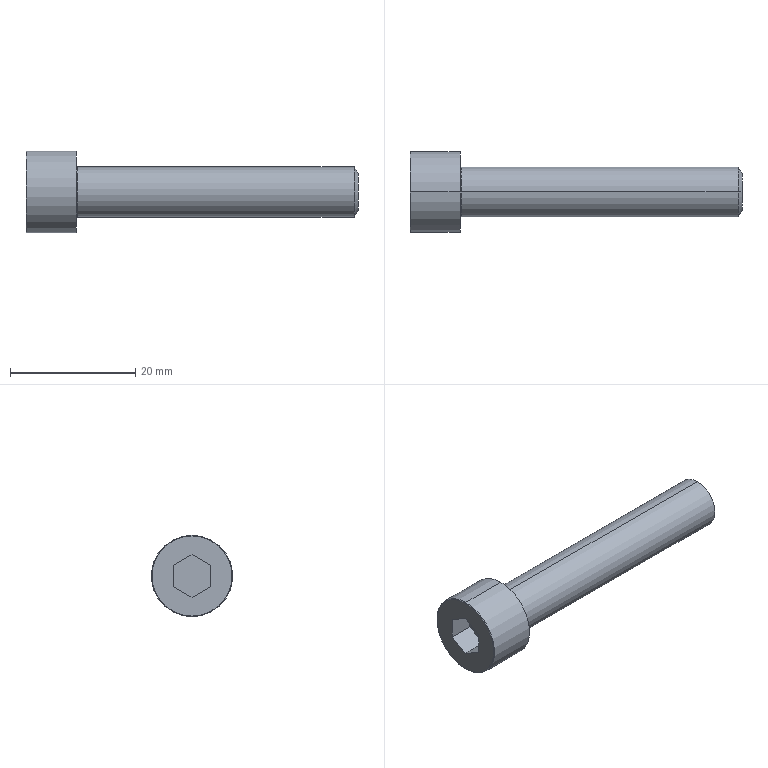Part | SolidWorks | features BlendCut 1, Cut 1, Fillet 1, LPattern 1, RevCut 1, Revolution 1 | 1 solid | 20 faces | box 53 x 13 x 13 mm | volume 3194 mm3 | plane 10 | torus 4 | cylinder 4 | cone 2 | commonest cylinder face diameters 8 x2 13 x2
STEP:
#1=CARTESIAN_POINT('',(0.,0.,6.4));
#2=VERTEX_POINT('',#1);
#3=CARTESIAN_POINT('',(0.,0.,-6.4));
#4=VERTEX_POINT('',#3);
#5=CARTESIAN_POINT('',(0.,0.,0.));
#6=DIRECTION('',(-1.,0.,0.));
#7=DIRECTION('',(0.,0.,-1.));
#8=AXIS2_PLACEMENT_3D('',#5,#6,#7);
#9=CIRCLE('',#8,6.4);
#10=EDGE_CURVE('',#2,#4,#9,.T.);
#11=ORIENTED_EDGE('',*,*,#10,.F.);
#12=CARTESIAN_POINT('',(0.1,0.,6.5));
#13=VERTEX_POINT('',#12);
#14=CARTESIAN_POINT('',(0.1,0.,6.4));
#15=DIRECTION('',(0.,1.,0.));
#16=DIRECTION('',(0.,0.,1.));
#17=AXIS2_PLACEMENT_3D('',#14,#15,#16);
#18=CIRCLE('',#17,0.1);
#19=EDGE_CURVE('',#2,#13,#18,.T.);
#20=ORIENTED_EDGE('',*,*,#19,.T.);
#21=CARTESIAN_POINT('',(0.1,0.,-6.5));
#22=VERTEX_POINT('',#21);
#23=CARTESIAN_POINT('',(0.1,0.,0.));
#24=DIRECTION('',(1.,0.,0.));
#25=DIRECTION('',(0.,0.,-1.));
#26=AXIS2_PLACEMENT_3D('',#23,#24,#25);
#27=CIRCLE('',#26,6.5);
#28=EDGE_CURVE('',#22,#13,#27,.T.);
#29=ORIENTED_EDGE('',*,*,#28,.F.);
#30=CARTESIAN_POINT('',(0.1,0.,-6.4));
#31=DIRECTION('',(0.,-1.,0.));
#32=DIRECTION('',(0.,0.,-1.));
#33=AXIS2_PLACEMENT_3D('',#30,#31,#32);
#34=CIRCLE('',#33,0.1);
#35=EDGE_CURVE('',#4,#22,#34,.T.);
#36=ORIENTED_EDGE('',*,*,#35,.F.);
#37=EDGE_LOOP('',(#11,#20,#29,#36));
#38=FACE_OUTER_BOUND('',#37,.T.);
#39=CARTESIAN_POINT('',(0.1,0.,0.));
#40=DIRECTION('',(1.,0.,0.));
#41=DIRECTION('',(0.,0.,-1.));
#42=AXIS2_PLACEMENT_3D('',#39,#40,#41);
#43=TOROIDAL_SURFACE('',#42,6.4,0.1);
#44=ADVANCED_FACE('',(#38),#43,.T.);
#45=CARTESIAN_POINT('',(53.,0.,2.917));
#46=VERTEX_POINT('',#45);
#47=CARTESIAN_POINT('',(53.,0.,-2.917));
#48=VERTEX_POINT('',#47);
#49=CARTESIAN_POINT('',(53.,0.,0.));
#50=DIRECTION('',(-1.,0.,0.));
#51=DIRECTION('',(0.,0.,1.));
#52=AXIS2_PLACEMENT_3D('',#49,#50,#51);
#53=CIRCLE('',#52,2.917);
#54=EDGE_CURVE('',#46,#48,#53,.T.);
#55=ORIENTED_EDGE('',*,*,#54,.T.);
#56=CARTESIAN_POINT('',(52.375,0.,-4.));
#57=VERTEX_POINT('',#56);
#58=CARTESIAN_POINT('',(52.375,0.,-4.));
#59=DIRECTION('',(-0.5,0.,-0.866));
#60=VECTOR('',#59,1000.);
#61=LINE('',#58,#60);
#62=EDGE_CURVE('',#48,#57,#61,.T.);
#63=ORIENTED_EDGE('',*,*,#62,.T.);
#64=CARTESIAN_POINT('',(52.375,0.,4.));
#65=VERTEX_POINT('',#64);
#66=CARTESIAN_POINT('',(52.375,0.,0.));
#67=DIRECTION('',(-1.,0.,0.));
#68=DIRECTION('',(0.,0.,1.));
#69=AXIS2_PLACEMENT_3D('',#66,#67,#68);
#70=CIRCLE('',#69,4.);
#71=EDGE_CURVE('',#65,#57,#70,.T.);
#72=ORIENTED_EDGE('',*,*,#71,.F.);
#73=CARTESIAN_POINT('',(52.375,0.,4.));
#74=DIRECTION('',(-0.5,0.,0.866));
#75=VECTOR('',#74,1000.);
#76=LINE('',#73,#75);
#77=EDGE_CURVE('',#46,#65,#76,.T.);
#78=ORIENTED_EDGE('',*,*,#77,.F.);
#79=EDGE_LOOP('',(#55,#63,#72,#78));
#80=FACE_OUTER_BOUND('',#79,.T.);
#81=CARTESIAN_POINT('',(52.375,0.,0.));
#82=DIRECTION('',(-1.,0.,0.));
#83=DIRECTION('',(0.,0.,1.));
#84=AXIS2_PLACEMENT_3D('',#81,#82,#83);
#85=CONICAL_SURFACE('',#84,4.,1.047);
#86=ADVANCED_FACE('',(#80),#85,.T.);
#87=CARTESIAN_POINT('',(8.,0.,-4.2));
#88=VERTEX_POINT('',#87);
#89=CARTESIAN_POINT('',(8.,0.,4.2));
#90=VERTEX_POINT('',#89);
#91=CARTESIAN_POINT('',(8.,0.,0.));
#92=DIRECTION('',(-1.,0.,0.));
#93=DIRECTION('',(0.,0.,1.));
#94=AXIS2_PLACEMENT_3D('',#91,#92,#93);
#95=CIRCLE('',#94,4.2);
#96=EDGE_CURVE('',#88,#90,#95,.T.);
#97=ORIENTED_EDGE('',*,*,#96,.F.);
#98=CARTESIAN_POINT('',(8.2,0.,-4.));
#99=VERTEX_POINT('',#98);
#100=CARTESIAN_POINT('',(8.2,0.,-4.2));
#101=DIRECTION('',(0.,1.,0.));
#102=DIRECTION('',(0.,0.,1.));
#103=AXIS2_PLACEMENT_3D('',#100,#101,#102);
#104=CIRCLE('',#103,0.2);
#105=EDGE_CURVE('',#88,#99,#104,.T.);
#106=ORIENTED_EDGE('',*,*,#105,.T.);
#107=CARTESIAN_POINT('',(8.2,0.,4.));
#108=VERTEX_POINT('',#107);
#109=CARTESIAN_POINT('',(8.2,0.,0.));
#110=DIRECTION('',(-1.,0.,0.));
#111=DIRECTION('',(0.,0.,1.));
#112=AXIS2_PLACEMENT_3D('',#109,#110,#111);
#113=CIRCLE('',#112,4.);
#114=EDGE_CURVE('',#99,#108,#113,.T.);
#115=ORIENTED_EDGE('',*,*,#114,.T.);
#116=CARTESIAN_POINT('',(8.2,0.,4.2));
#117=DIRECTION('',(0.,-1.,0.));
#118=DIRECTION('',(0.,0.,-1.));
#119=AXIS2_PLACEMENT_3D('',#116,#117,#118);
#120=CIRCLE('',#119,0.2);
#121=EDGE_CURVE('',#90,#108,#120,.T.);
#122=ORIENTED_EDGE('',*,*,#121,.F.);
#123=EDGE_LOOP('',(#97,#106,#115,#122));
#124=FACE_OUTER_BOUND('',#123,.T.);
#125=CARTESIAN_POINT('',(8.2,0.,0.));
#126=DIRECTION('',(-1.,0.,0.));
#127=DIRECTION('',(0.,0.,1.));
#128=AXIS2_PLACEMENT_3D('',#125,#126,#127);
#129=TOROIDAL_SURFACE('',#128,4.2,0.2);
#130=ADVANCED_FACE('',(#124),#129,.F.);
#131=CARTESIAN_POINT('',(8.,0.,6.5));
#132=VERTEX_POINT('',#131);
#133=CARTESIAN_POINT('',(8.,0.,-6.5));
#134=VERTEX_POINT('',#133);
#135=CARTESIAN_POINT('',(8.,0.,0.));
#136=DIRECTION('',(-1.,0.,0.));
#137=DIRECTION('',(0.,0.,1.));
#138=AXIS2_PLACEMENT_3D('',#135,#136,#137);
#139=CIRCLE('',#138,6.5);
#140=EDGE_CURVE('',#132,#134,#139,.T.);
#141=ORIENTED_EDGE('',*,*,#140,.T.);
#142=CARTESIAN_POINT('',(0.,0.,-6.5));
#143=DIRECTION('',(-1.,0.,0.));
#144=VECTOR('',#143,1000.);
#145=LINE('',#142,#144);
#146=EDGE_CURVE('',#134,#22,#145,.T.);
#147=ORIENTED_EDGE('',*,*,#146,.T.);
#148=ORIENTED_EDGE('',*,*,#28,.T.);
#149=CARTESIAN_POINT('',(0.,0.,6.5));
#150=DIRECTION('',(-1.,0.,0.));
#151=VECTOR('',#150,1000.);
#152=LINE('',#149,#151);
#153=EDGE_CURVE('',#132,#13,#152,.T.);
#154=ORIENTED_EDGE('',*,*,#153,.F.);
#155=EDGE_LOOP('',(#141,#147,#148,#154));
#156=FACE_OUTER_BOUND('',#155,.T.);
#157=CARTESIAN_POINT('',(0.,0.,0.));
#158=DIRECTION('',(-1.,0.,0.));
#159=DIRECTION('',(0.,0.,1.));
#160=AXIS2_PLACEMENT_3D('',#157,#158,#159);
#161=CYLINDRICAL_SURFACE('',#160,6.5);
#162=ADVANCED_FACE('',(#156),#161,.T.);
#163=ORIENTED_EDGE('',*,*,#71,.T.);
#164=CARTESIAN_POINT('',(0.,0.,-4.));
#165=DIRECTION('',(-1.,0.,0.));
#166=VECTOR('',#165,1000.);
#167=LINE('',#164,#166);
#168=EDGE_CURVE('',#57,#99,#167,.T.);
#169=ORIENTED_EDGE('',*,*,#168,.T.);
#170=CARTESIAN_POINT('',(8.2,0.,0.));
#171=DIRECTION('',(-1.,0.,0.));
#172=DIRECTION('',(0.,0.,1.));
#173=AXIS2_PLACEMENT_3D('',#170,#171,#172);
#174=CIRCLE('',#173,4.);
#175=EDGE_CURVE('',#108,#99,#174,.T.);
#176=ORIENTED_EDGE('',*,*,#175,.F.);
#177=CARTESIAN_POINT('',(0.,0.,4.));
#178=DIRECTION('',(-1.,0.,0.));
#179=VECTOR('',#178,1000.);
#180=LINE('',#177,#179);
#181=EDGE_CURVE('',#65,#108,#180,.T.);
#182=ORIENTED_EDGE('',*,*,#181,.F.);
#183=EDGE_LOOP('',(#163,#169,#176,#182));
#184=FACE_OUTER_BOUND('',#183,.T.);
#185=CARTESIAN_POINT('',(0.,0.,0.));
#186=DIRECTION('',(-1.,0.,0.));
#187=DIRECTION('',(0.,0.,1.));
#188=AXIS2_PLACEMENT_3D('',#185,#186,#187);
#189=CYLINDRICAL_SURFACE('',#188,4.);
#190=ADVANCED_FACE('',(#184),#189,.T.);
#191=ORIENTED_EDGE('',*,*,#168,.F.);
#192=CARTESIAN_POINT('',(52.375,0.,0.));
#193=DIRECTION('',(-1.,0.,0.));
#194=DIRECTION('',(0.,0.,1.));
#195=AXIS2_PLACEMENT_3D('',#192,#193,#194);
#196=CIRCLE('',#195,4.);
#197=EDGE_CURVE('',#57,#65,#196,.T.);
#198=ORIENTED_EDGE('',*,*,#197,.T.);
#199=ORIENTED_EDGE('',*,*,#181,.T.);
#200=ORIENTED_EDGE('',*,*,#114,.F.);
#201=EDGE_LOOP('',(#191,#198,#199,#200));
#202=FACE_OUTER_BOUND('',#201,.T.);
#203=CARTESIAN_POINT('',(0.,0.,0.));
#204=DIRECTION('',(-1.,0.,0.));
#205=DIRECTION('',(0.,0.,1.));
#206=AXIS2_PLACEMENT_3D('',#203,#204,#205);
#207=CYLINDRICAL_SURFACE('',#206,4.);
#208=ADVANCED_FACE('',(#202),#207,.T.);
#209=CARTESIAN_POINT('',(0.,0.,0.));
#210=DIRECTION('',(-1.,0.,0.));
#211=DIRECTION('',(0.,0.,-1.));
#212=AXIS2_PLACEMENT_3D('',#209,#210,#211);
#213=CIRCLE('',#212,6.4);
#214=EDGE_CURVE('',#4,#2,#213,.T.);
#215=ORIENTED_EDGE('',*,*,#214,.T.);
#216=ORIENTED_EDGE('',*,*,#10,.T.);
#217=EDGE_LOOP('',(#215,#216));
#218=FACE_OUTER_BOUND('',#217,.T.);
#219=CARTESIAN_POINT('',(0.,0.,3.43));
#220=VERTEX_POINT('',#219);
#221=CARTESIAN_POINT('',(0.,2.97,1.715));
#222=VERTEX_POINT('',#221);
#223=CARTESIAN_POINT('',(0.,0.,3.43));
#224=DIRECTION('',(0.,0.866,-0.5));
#225=VECTOR('',#224,1000.);
#226=LINE('',#223,#225);
#227=EDGE_CURVE('',#220,#222,#226,.T.);
#228=ORIENTED_EDGE('',*,*,#227,.F.);
#229=CARTESIAN_POINT('',(0.,-2.97,1.715));
#230=VERTEX_POINT('',#229);
#231=CARTESIAN_POINT('',(0.,-2.97,1.715));
#232=DIRECTION('',(0.,0.866,0.5));
#233=VECTOR('',#232,1000.);
#234=LINE('',#231,#233);
#235=EDGE_CURVE('',#230,#220,#234,.T.);
#236=ORIENTED_EDGE('',*,*,#235,.F.);
#237=CARTESIAN_POINT('',(0.,-2.97,-1.715));
#238=VERTEX_POINT('',#237);
#239=CARTESIAN_POINT('',(0.,-2.97,-1.715));
#240=DIRECTION('',(0.,0.,1.));
#241=VECTOR('',#240,1000.);
#242=LINE('',#239,#241);
#243=EDGE_CURVE('',#238,#230,#242,.T.);
#244=ORIENTED_EDGE('',*,*,#243,.F.);
#245=CARTESIAN_POINT('',(0.,0.,-3.43));
#246=VERTEX_POINT('',#245);
#247=CARTESIAN_POINT('',(0.,0.,-3.43));
#248=DIRECTION('',(0.,-0.866,0.5));
#249=VECTOR('',#248,1000.);
#250=LINE('',#247,#249);
#251=EDGE_CURVE('',#246,#238,#250,.T.);
#252=ORIENTED_EDGE('',*,*,#251,.F.);
#253=CARTESIAN_POINT('',(0.,2.97,-1.715));
#254=VERTEX_POINT('',#253);
#255=CARTESIAN_POINT('',(0.,2.97,-1.715));
#256=DIRECTION('',(0.,-0.866,-0.5));
#257=VECTOR('',#256,1000.);
#258=LINE('',#255,#257);
#259=EDGE_CURVE('',#254,#246,#258,.T.);
#260=ORIENTED_EDGE('',*,*,#259,.F.);
#261=CARTESIAN_POINT('',(0.,2.97,1.715));
#262=DIRECTION('',(0.,0.,-1.));
#263=VECTOR('',#262,1000.);
#264=LINE('',#261,#263);
#265=EDGE_CURVE('',#222,#254,#264,.T.);
#266=ORIENTED_EDGE('',*,*,#265,.F.);
#267=EDGE_LOOP('',(#228,#236,#244,#252,#260,#266));
#268=FACE_BOUND('',#267,.T.);
#269=CARTESIAN_POINT('',(0.,0.,0.));
#270=DIRECTION('',(1.,0.,0.));
#271=DIRECTION('',(0.,0.,-1.));
#272=AXIS2_PLACEMENT_3D('',#269,#270,#271);
#273=PLANE('',#272);
#274=ADVANCED_FACE('',(#218,#268),#273,.F.);
#275=ORIENTED_EDGE('',*,*,#146,.F.);
#276=CARTESIAN_POINT('',(8.,0.,0.));
#277=DIRECTION('',(-1.,0.,0.));
#278=DIRECTION('',(0.,0.,1.));
#279=AXIS2_PLACEMENT_3D('',#276,#277,#278);
#280=CIRCLE('',#279,6.5);
#281=EDGE_CURVE('',#134,#132,#280,.T.);
#282=ORIENTED_EDGE('',*,*,#281,.T.);
#283=ORIENTED_EDGE('',*,*,#153,.T.);
#284=CARTESIAN_POINT('',(0.1,0.,0.));
#285=DIRECTION('',(1.,0.,0.));
#286=DIRECTION('',(0.,0.,-1.));
#287=AXIS2_PLACEMENT_3D('',#284,#285,#286);
#288=CIRCLE('',#287,6.5);
#289=EDGE_CURVE('',#13,#22,#288,.T.);
#290=ORIENTED_EDGE('',*,*,#289,.T.);
#291=EDGE_LOOP('',(#275,#282,#283,#290));
#292=FACE_OUTER_BOUND('',#291,.T.);
#293=CARTESIAN_POINT('',(0.,0.,0.));
#294=DIRECTION('',(-1.,0.,0.));
#295=DIRECTION('',(0.,0.,1.));
#296=AXIS2_PLACEMENT_3D('',#293,#294,#295);
#297=CYLINDRICAL_SURFACE('',#296,6.5);
#298=ADVANCED_FACE('',(#292),#297,.T.);
#299=ORIENTED_EDGE('',*,*,#140,.F.);
#300=ORIENTED_EDGE('',*,*,#281,.F.);
#301=EDGE_LOOP('',(#299,#300));
#302=FACE_OUTER_BOUND('',#301,.T.);
#303=CARTESIAN_POINT('',(8.,0.,0.));
#304=DIRECTION('',(-1.,0.,0.));
#305=DIRECTION('',(0.,0.,1.));
#306=AXIS2_PLACEMENT_3D('',#303,#304,#305);
#307=CIRCLE('',#306,4.2);
#308=EDGE_CURVE('',#90,#88,#307,.T.);
#309=ORIENTED_EDGE('',*,*,#308,.T.);
#310=ORIENTED_EDGE('',*,*,#96,.T.);
#311=EDGE_LOOP('',(#309,#310));
#312=FACE_BOUND('',#311,.T.);
#313=CARTESIAN_POINT('',(8.,6.5,0.));
#314=DIRECTION('',(-1.,0.,0.));
#315=DIRECTION('',(0.,0.,1.));
#316=AXIS2_PLACEMENT_3D('',#313,#314,#315);
#317=PLANE('',#316);
#318=ADVANCED_FACE('',(#302,#312),#317,.F.);
#319=ORIENTED_EDGE('',*,*,#105,.F.);
#320=ORIENTED_EDGE('',*,*,#308,.F.);
#321=ORIENTED_EDGE('',*,*,#121,.T.);
#322=ORIENTED_EDGE('',*,*,#175,.T.);
#323=EDGE_LOOP('',(#319,#320,#321,#322));
#324=FACE_OUTER_BOUND('',#323,.T.);
#325=CARTESIAN_POINT('',(8.2,0.,0.));
#326=DIRECTION('',(-1.,0.,0.));
#327=DIRECTION('',(0.,0.,1.));
#328=AXIS2_PLACEMENT_3D('',#325,#326,#327);
#329=TOROIDAL_SURFACE('',#328,4.2,0.2);
#330=ADVANCED_FACE('',(#324),#329,.F.);
#331=ORIENTED_EDGE('',*,*,#235,.T.);
#332=CARTESIAN_POINT('',(4.,0.,3.43));
#333=VERTEX_POINT('',#332);
#334=CARTESIAN_POINT('',(4.,0.,3.43));
#335=DIRECTION('',(-1.,0.,0.));
#336=VECTOR('',#335,1000.);
#337=LINE('',#334,#336);
#338=EDGE_CURVE('',#333,#220,#337,.T.);
#339=ORIENTED_EDGE('',*,*,#338,.F.);
#340=CARTESIAN_POINT('',(4.,-2.97,1.715));
#341=VERTEX_POINT('',#340);
#342=CARTESIAN_POINT('',(4.,-2.97,1.715));
#343=DIRECTION('',(0.,0.866,0.5));
#344=VECTOR('',#343,1000.);
#345=LINE('',#342,#344);
#346=EDGE_CURVE('',#341,#333,#345,.T.);
#347=ORIENTED_EDGE('',*,*,#346,.F.);
#348=CARTESIAN_POINT('',(4.,-2.97,1.715));
#349=DIRECTION('',(-1.,0.,0.));
#350=VECTOR('',#349,1000.);
#351=LINE('',#348,#350);
#352=EDGE_CURVE('',#341,#230,#351,.T.);
#353=ORIENTED_EDGE('',*,*,#352,.T.);
#354=EDGE_LOOP('',(#331,#339,#347,#353));
#355=FACE_OUTER_BOUND('',#354,.T.);
#356=CARTESIAN_POINT('',(4.,-2.97,1.715));
#357=DIRECTION('',(0.,-0.5,0.866));
#358=DIRECTION('',(0.,-0.866,-0.5));
#359=AXIS2_PLACEMENT_3D('',#356,#357,#358);
#360=PLANE('',#359);
#361=ADVANCED_FACE('',(#355),#360,.F.);
#362=ORIENTED_EDGE('',*,*,#243,.T.);
#363=ORIENTED_EDGE('',*,*,#352,.F.);
#364=CARTESIAN_POINT('',(4.,-2.97,-1.715));
#365=VERTEX_POINT('',#364);
#366=CARTESIAN_POINT('',(4.,-2.97,-1.715));
#367=DIRECTION('',(0.,0.,1.));
#368=VECTOR('',#367,1000.);
#369=LINE('',#366,#368);
#370=EDGE_CURVE('',#365,#341,#369,.T.);
#371=ORIENTED_EDGE('',*,*,#370,.F.);
#372=CARTESIAN_POINT('',(4.,-2.97,-1.715));
#373=DIRECTION('',(-1.,0.,0.));
#374=VECTOR('',#373,1000.);
#375=LINE('',#372,#374);
#376=EDGE_CURVE('',#365,#238,#375,.T.);
#377=ORIENTED_EDGE('',*,*,#376,.T.);
#378=EDGE_LOOP('',(#362,#363,#371,#377));
#379=FACE_OUTER_BOUND('',#378,.T.);
#380=CARTESIAN_POINT('',(4.,-2.97,-1.715));
#381=DIRECTION('',(0.,-1.,0.));
#382=DIRECTION('',(0.,0.,-1.));
#383=AXIS2_PLACEMENT_3D('',#380,#381,#382);
#384=PLANE('',#383);
#385=ADVANCED_FACE('',(#379),#384,.F.);
#386=ORIENTED_EDGE('',*,*,#251,.T.);
#387=ORIENTED_EDGE('',*,*,#376,.F.);
#388=CARTESIAN_POINT('',(4.,0.,-3.43));
#389=VERTEX_POINT('',#388);
#390=CARTESIAN_POINT('',(4.,0.,-3.43));
#391=DIRECTION('',(0.,-0.866,0.5));
#392=VECTOR('',#391,1000.);
#393=LINE('',#390,#392);
#394=EDGE_CURVE('',#389,#365,#393,.T.);
#395=ORIENTED_EDGE('',*,*,#394,.F.);
#396=CARTESIAN_POINT('',(4.,0.,-3.43));
#397=DIRECTION('',(-1.,0.,0.));
#398=VECTOR('',#397,1000.);
#399=LINE('',#396,#398);
#400=EDGE_CURVE('',#389,#246,#399,.T.);
#401=ORIENTED_EDGE('',*,*,#400,.T.);
#402=EDGE_LOOP('',(#386,#387,#395,#401));
#403=FACE_OUTER_BOUND('',#402,.T.);
#404=CARTESIAN_POINT('',(4.,0.,-3.43));
#405=DIRECTION('',(0.,-0.5,-0.866));
#406=DIRECTION('',(0.,0.866,-0.5));
#407=AXIS2_PLACEMENT_3D('',#404,#405,#406);
#408=PLANE('',#407);
#409=ADVANCED_FACE('',(#403),#408,.F.);
#410=ORIENTED_EDGE('',*,*,#259,.T.);
#411=ORIENTED_EDGE('',*,*,#400,.F.);
#412=CARTESIAN_POINT('',(4.,2.97,-1.715));
#413=VERTEX_POINT('',#412);
#414=CARTESIAN_POINT('',(4.,2.97,-1.715));
#415=DIRECTION('',(0.,-0.866,-0.5));
#416=VECTOR('',#415,1000.);
#417=LINE('',#414,#416);
#418=EDGE_CURVE('',#413,#389,#417,.T.);
#419=ORIENTED_EDGE('',*,*,#418,.F.);
#420=CARTESIAN_POINT('',(4.,2.97,-1.715));
#421=DIRECTION('',(-1.,0.,0.));
#422=VECTOR('',#421,1000.);
#423=LINE('',#420,#422);
#424=EDGE_CURVE('',#413,#254,#423,.T.);
#425=ORIENTED_EDGE('',*,*,#424,.T.);
#426=EDGE_LOOP('',(#410,#411,#419,#425));
#427=FACE_OUTER_BOUND('',#426,.T.);
#428=CARTESIAN_POINT('',(4.,2.97,-1.715));
#429=DIRECTION('',(0.,0.5,-0.866));
#430=DIRECTION('',(0.,0.866,0.5));
#431=AXIS2_PLACEMENT_3D('',#428,#429,#430);
#432=PLANE('',#431);
#433=ADVANCED_FACE('',(#427),#432,.F.);
#434=ORIENTED_EDGE('',*,*,#265,.T.);
#435=ORIENTED_EDGE('',*,*,#424,.F.);
#436=CARTESIAN_POINT('',(4.,2.97,1.715));
#437=VERTEX_POINT('',#436);
#438=CARTESIAN_POINT('',(4.,2.97,1.715));
#439=DIRECTION('',(0.,0.,-1.));
#440=VECTOR('',#439,1000.);
#441=LINE('',#438,#440);
#442=EDGE_CURVE('',#437,#413,#441,.T.);
#443=ORIENTED_EDGE('',*,*,#442,.F.);
#444=CARTESIAN_POINT('',(4.,2.97,1.715));
#445=DIRECTION('',(-1.,0.,0.));
#446=VECTOR('',#445,1000.);
#447=LINE('',#444,#446);
#448=EDGE_CURVE('',#437,#222,#447,.T.);
#449=ORIENTED_EDGE('',*,*,#448,.T.);
#450=EDGE_LOOP('',(#434,#435,#443,#449));
#451=FACE_OUTER_BOUND('',#450,.T.);
#452=CARTESIAN_POINT('',(4.,2.97,1.715));
#453=DIRECTION('',(0.,1.,0.));
#454=DIRECTION('',(0.,0.,1.));
#455=AXIS2_PLACEMENT_3D('',#452,#453,#454);
#456=PLANE('',#455);
#457=ADVANCED_FACE('',(#451),#456,.F.);
#458=ORIENTED_EDGE('',*,*,#227,.T.);
#459=ORIENTED_EDGE('',*,*,#448,.F.);
#460=CARTESIAN_POINT('',(4.,0.,3.43));
#461=DIRECTION('',(0.,0.866,-0.5));
#462=VECTOR('',#461,1000.);
#463=LINE('',#460,#462);
#464=EDGE_CURVE('',#333,#437,#463,.T.);
#465=ORIENTED_EDGE('',*,*,#464,.F.);
#466=ORIENTED_EDGE('',*,*,#338,.T.);
#467=EDGE_LOOP('',(#458,#459,#465,#466));
#468=FACE_OUTER_BOUND('',#467,.T.);
#469=CARTESIAN_POINT('',(4.,0.,3.43));
#470=DIRECTION('',(0.,0.5,0.866));
#471=DIRECTION('',(0.,-0.866,0.5));
#472=AXIS2_PLACEMENT_3D('',#469,#470,#471);
#473=PLANE('',#472);
#474=ADVANCED_FACE('',(#468),#473,.F.);
#475=ORIENTED_EDGE('',*,*,#346,.T.);
#476=ORIENTED_EDGE('',*,*,#464,.T.);
#477=ORIENTED_EDGE('',*,*,#442,.T.);
#478=ORIENTED_EDGE('',*,*,#418,.T.);
#479=ORIENTED_EDGE('',*,*,#394,.T.);
#480=ORIENTED_EDGE('',*,*,#370,.T.);
#481=EDGE_LOOP('',(#475,#476,#477,#478,#479,#480));
#482=FACE_OUTER_BOUND('',#481,.T.);
#483=CARTESIAN_POINT('',(4.,-2.97,1.715));
#484=DIRECTION('',(1.,0.,0.));
#485=DIRECTION('',(0.,0.,-1.));
#486=AXIS2_PLACEMENT_3D('',#483,#484,#485);
#487=PLANE('',#486);
#488=ADVANCED_FACE('',(#482),#487,.F.);
#489=ORIENTED_EDGE('',*,*,#62,.F.);
#490=CARTESIAN_POINT('',(53.,0.,0.));
#491=DIRECTION('',(-1.,0.,0.));
#492=DIRECTION('',(0.,0.,1.));
#493=AXIS2_PLACEMENT_3D('',#490,#491,#492);
#494=CIRCLE('',#493,2.917);
#495=EDGE_CURVE('',#48,#46,#494,.T.);
#496=ORIENTED_EDGE('',*,*,#495,.T.);
#497=ORIENTED_EDGE('',*,*,#77,.T.);
#498=ORIENTED_EDGE('',*,*,#197,.F.);
#499=EDGE_LOOP('',(#489,#496,#497,#498));
#500=FACE_OUTER_BOUND('',#499,.T.);
#501=CARTESIAN_POINT('',(52.375,0.,0.));
#502=DIRECTION('',(-1.,0.,0.));
#503=DIRECTION('',(0.,0.,1.));
#504=AXIS2_PLACEMENT_3D('',#501,#502,#503);
#505=CONICAL_SURFACE('',#504,4.,1.047);
#506=ADVANCED_FACE('',(#500),#505,.T.);
#507=ORIENTED_EDGE('',*,*,#54,.F.);
#508=ORIENTED_EDGE('',*,*,#495,.F.);
#509=EDGE_LOOP('',(#507,#508));
#510=FACE_OUTER_BOUND('',#509,.T.);
#511=CARTESIAN_POINT('',(53.,4.,0.));
#512=DIRECTION('',(-1.,0.,0.));
#513=DIRECTION('',(0.,0.,1.));
#514=AXIS2_PLACEMENT_3D('',#511,#512,#513);
#515=PLANE('',#514);
#516=ADVANCED_FACE('',(#510),#515,.F.);
#517=ORIENTED_EDGE('',*,*,#19,.F.);
#518=ORIENTED_EDGE('',*,*,#214,.F.);
#519=ORIENTED_EDGE('',*,*,#35,.T.);
#520=ORIENTED_EDGE('',*,*,#289,.F.);
#521=EDGE_LOOP('',(#517,#518,#519,#520));
#522=FACE_OUTER_BOUND('',#521,.T.);
#523=CARTESIAN_POINT('',(0.1,0.,0.));
#524=DIRECTION('',(1.,0.,0.));
#525=DIRECTION('',(0.,0.,-1.));
#526=AXIS2_PLACEMENT_3D('',#523,#524,#525);
#527=TOROIDAL_SURFACE('',#526,6.4,0.1);
#528=ADVANCED_FACE('',(#522),#527,.T.);
#529=CLOSED_SHELL('',(#44,#86,#130,#162,#190,#208,#274,#298,#318,#330,#361,#385,#409,#433,#457,#474,#488,#506,#516,#528));
#530=MANIFOLD_SOLID_BREP('',#529);
#531=CARTESIAN_POINT('',(0.,0.,0.));
#532=DIRECTION('',(0.,0.,1.));
#533=DIRECTION('',(1.,0.,0.));
#534=AXIS2_PLACEMENT_3D('',#531,#532,#533);
#535=(LENGTH_UNIT()NAMED_UNIT(*)SI_UNIT(.MILLI.,.METRE.));
#536=UNCERTAINTY_MEASURE_WITH_UNIT(LENGTH_MEASURE(0.00001),#535,'','');
#537=(NAMED_UNIT(*)PLANE_ANGLE_UNIT()SI_UNIT($,.RADIAN.));
#538=(NAMED_UNIT(*)SI_UNIT($,.STERADIAN.)SOLID_ANGLE_UNIT());
#539=(GEOMETRIC_REPRESENTATION_CONTEXT(3)GLOBAL_UNCERTAINTY_ASSIGNED_CONTEXT((#536))GLOBAL_UNIT_ASSIGNED_CONTEXT((#535,#537,#538))REPRESENTATION_CONTEXT('',''));
#540=ADVANCED_BREP_SHAPE_REPRESENTATION('',(#530,#534),#539);